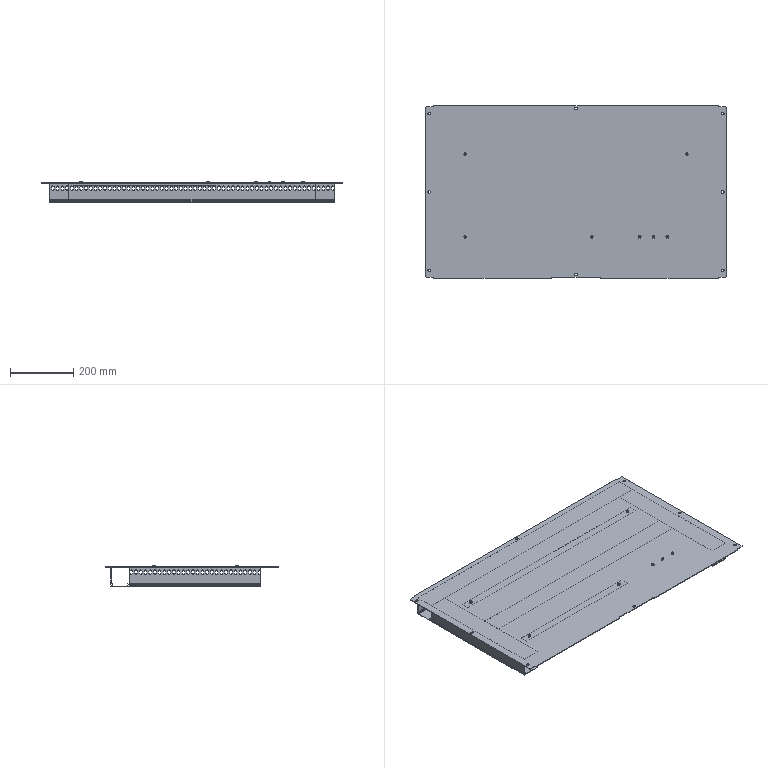Part | SolidWorks | 7 solids | 1696 faces | box 950 x 544 x 66 mm | volume 1696840 mm3 | plane 932 | cylinder 764 | commonest cylinder face diameters 8 x672 6.5 x24 5.5 x20 5 x14 6 x12 1 x8